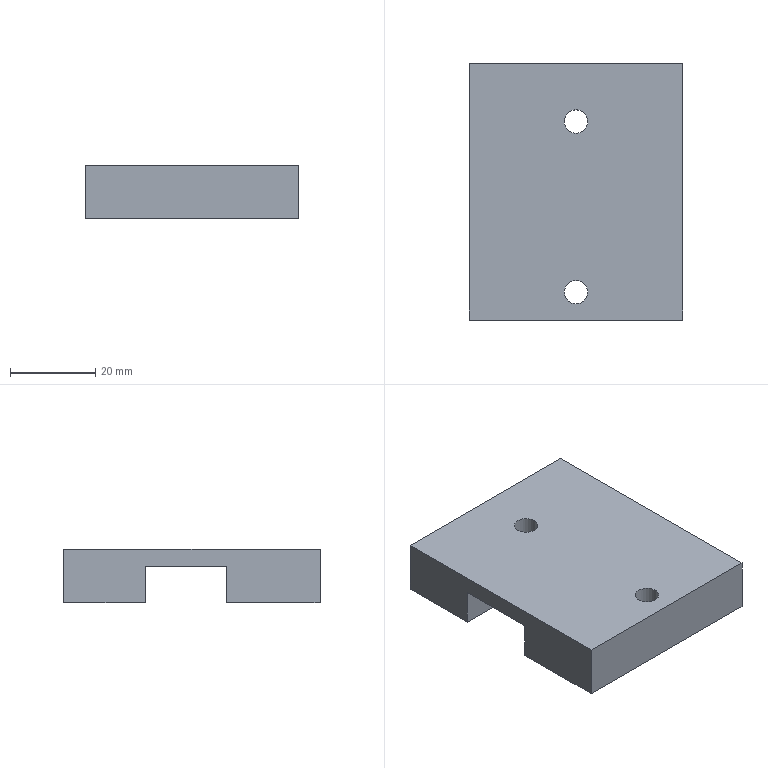Part | STEP file | 1 solid | 16 faces | box 50 x 60 x 12.5 mm | volume 28207 mm3 | plane 12 | cylinder 4 | commonest cylinder face diameters 5.5 x2 10 x2
STEP:
#1=CARTESIAN_POINT('',(0.,0.,0.));
#2=DIRECTION('',(0.,0.,1.));
#3=DIRECTION('',(1.,0.,0.));
#4=AXIS2_PLACEMENT_3D('',#1,#2,#3);
#5=CARTESIAN_POINT('',(-25.,0.,12.5));
#6=VERTEX_POINT('',#5);
#7=CARTESIAN_POINT('',(25.,0.,12.5));
#8=VERTEX_POINT('',#7);
#9=CARTESIAN_POINT('',(-25.,0.,12.5));
#10=DIRECTION('',(1.,0.,0.));
#11=VECTOR('',#10,1.);
#12=LINE('',#9,#11);
#13=CARTESIAN_POINT('',(0.,0.,12.5));
#14=DIRECTION('',(0.,0.,1.));
#15=DIRECTION('',(1.,0.,0.));
#16=AXIS2_PLACEMENT_3D('',#13,#14,#15);
#17=PLANE('',#16);
#18=CARTESIAN_POINT('',(-25.,0.));
#19=DIRECTION('',(1.,0.));
#20=VECTOR('',#19,1.);
#21=LINE('',#18,#20);
#22=(GEOMETRIC_REPRESENTATION_CONTEXT(2)PARAMETRIC_REPRESENTATION_CONTEXT()REPRESENTATION_CONTEXT('',''));
#23=DEFINITIONAL_REPRESENTATION('',(#21),#22);
#24=PCURVE('',#17,#23);
#25=CARTESIAN_POINT('',(0.,0.,0.));
#26=DIRECTION('',(0.,-1.,0.));
#27=DIRECTION('',(0.,0.,-1.));
#28=AXIS2_PLACEMENT_3D('',#25,#26,#27);
#29=PLANE('',#28);
#30=CARTESIAN_POINT('',(-12.5,-25.));
#31=DIRECTION('',(0.,1.));
#32=VECTOR('',#31,1.);
#33=LINE('',#30,#32);
#34=(GEOMETRIC_REPRESENTATION_CONTEXT(2)PARAMETRIC_REPRESENTATION_CONTEXT()REPRESENTATION_CONTEXT('',''));
#35=DEFINITIONAL_REPRESENTATION('',(#33),#34);
#36=PCURVE('',#29,#35);
#37=SURFACE_CURVE('',#12,(#24,#36),.PCURVE_S1.);
#38=EDGE_CURVE('',#6,#8,#37,.T.);
#39=ORIENTED_EDGE('',*,*,#38,.T.);
#40=CARTESIAN_POINT('',(25.,60.,12.5));
#41=VERTEX_POINT('',#40);
#42=CARTESIAN_POINT('',(25.,60.,12.5));
#43=DIRECTION('',(0.,-1.,0.));
#44=VECTOR('',#43,1.);
#45=LINE('',#42,#44);
#46=CARTESIAN_POINT('',(25.,60.));
#47=DIRECTION('',(0.,-1.));
#48=VECTOR('',#47,1.);
#49=LINE('',#46,#48);
#50=(GEOMETRIC_REPRESENTATION_CONTEXT(2)PARAMETRIC_REPRESENTATION_CONTEXT()REPRESENTATION_CONTEXT('',''));
#51=DEFINITIONAL_REPRESENTATION('',(#49),#50);
#52=PCURVE('',#17,#51);
#53=CARTESIAN_POINT('',(25.,0.,0.));
#54=DIRECTION('',(1.,0.,0.));
#55=DIRECTION('',(0.,0.,-1.));
#56=AXIS2_PLACEMENT_3D('',#53,#54,#55);
#57=PLANE('',#56);
#58=CARTESIAN_POINT('',(-12.5,60.));
#59=DIRECTION('',(0.,-1.));
#60=VECTOR('',#59,1.);
#61=LINE('',#58,#60);
#62=(GEOMETRIC_REPRESENTATION_CONTEXT(2)PARAMETRIC_REPRESENTATION_CONTEXT()REPRESENTATION_CONTEXT('',''));
#63=DEFINITIONAL_REPRESENTATION('',(#61),#62);
#64=PCURVE('',#57,#63);
#65=SURFACE_CURVE('',#45,(#52,#64),.PCURVE_S1.);
#66=EDGE_CURVE('',#41,#8,#65,.T.);
#67=ORIENTED_EDGE('',*,*,#66,.F.);
#68=CARTESIAN_POINT('',(-25.,60.,12.5));
#69=VERTEX_POINT('',#68);
#70=CARTESIAN_POINT('',(-25.,60.,12.5));
#71=DIRECTION('',(1.,0.,0.));
#72=VECTOR('',#71,1.);
#73=LINE('',#70,#72);
#74=CARTESIAN_POINT('',(-25.,60.));
#75=DIRECTION('',(1.,0.));
#76=VECTOR('',#75,1.);
#77=LINE('',#74,#76);
#78=(GEOMETRIC_REPRESENTATION_CONTEXT(2)PARAMETRIC_REPRESENTATION_CONTEXT()REPRESENTATION_CONTEXT('',''));
#79=DEFINITIONAL_REPRESENTATION('',(#77),#78);
#80=PCURVE('',#17,#79);
#81=CARTESIAN_POINT('',(0.,60.,0.));
#82=DIRECTION('',(0.,1.,0.));
#83=DIRECTION('',(0.,0.,1.));
#84=AXIS2_PLACEMENT_3D('',#81,#82,#83);
#85=PLANE('',#84);
#86=CARTESIAN_POINT('',(12.5,-25.));
#87=DIRECTION('',(0.,1.));
#88=VECTOR('',#87,1.);
#89=LINE('',#86,#88);
#90=(GEOMETRIC_REPRESENTATION_CONTEXT(2)PARAMETRIC_REPRESENTATION_CONTEXT()REPRESENTATION_CONTEXT('',''));
#91=DEFINITIONAL_REPRESENTATION('',(#89),#90);
#92=PCURVE('',#85,#91);
#93=SURFACE_CURVE('',#73,(#80,#92),.PCURVE_S1.);
#94=EDGE_CURVE('',#69,#41,#93,.T.);
#95=ORIENTED_EDGE('',*,*,#94,.F.);
#96=CARTESIAN_POINT('',(-25.,60.,12.5));
#97=DIRECTION('',(0.,-1.,0.));
#98=VECTOR('',#97,1.);
#99=LINE('',#96,#98);
#100=CARTESIAN_POINT('',(-25.,60.));
#101=DIRECTION('',(0.,-1.));
#102=VECTOR('',#101,1.);
#103=LINE('',#100,#102);
#104=(GEOMETRIC_REPRESENTATION_CONTEXT(2)PARAMETRIC_REPRESENTATION_CONTEXT()REPRESENTATION_CONTEXT('',''));
#105=DEFINITIONAL_REPRESENTATION('',(#103),#104);
#106=PCURVE('',#17,#105);
#107=CARTESIAN_POINT('',(-25.,0.,0.));
#108=DIRECTION('',(1.,0.,0.));
#109=DIRECTION('',(0.,0.,-1.));
#110=AXIS2_PLACEMENT_3D('',#107,#108,#109);
#111=PLANE('',#110);
#112=CARTESIAN_POINT('',(-12.5,60.));
#113=DIRECTION('',(0.,-1.));
#114=VECTOR('',#113,1.);
#115=LINE('',#112,#114);
#116=(GEOMETRIC_REPRESENTATION_CONTEXT(2)PARAMETRIC_REPRESENTATION_CONTEXT()REPRESENTATION_CONTEXT('',''));
#117=DEFINITIONAL_REPRESENTATION('',(#115),#116);
#118=PCURVE('',#111,#117);
#119=SURFACE_CURVE('',#99,(#106,#118),.PCURVE_S1.);
#120=EDGE_CURVE('',#69,#6,#119,.T.);
#121=ORIENTED_EDGE('',*,*,#120,.T.);
#122=EDGE_LOOP('',(#39,#67,#95,#121));
#123=FACE_BOUND('',#122,.T.);
#124=CARTESIAN_POINT('',(0.,43.75,12.5));
#125=VERTEX_POINT('',#124);
#126=CARTESIAN_POINT('',(0.,46.5,12.5));
#127=DIRECTION('',(0.,0.,1.));
#128=DIRECTION('',(1.,0.,0.));
#129=AXIS2_PLACEMENT_3D('',#126,#127,#128);
#130=CIRCLE('',#129,2.75);
#131=CARTESIAN_POINT('',(0.,46.5));
#132=DIRECTION('',(1.,0.));
#133=AXIS2_PLACEMENT_2D('',#131,#132);
#134=CIRCLE('',#133,2.75);
#135=(GEOMETRIC_REPRESENTATION_CONTEXT(2)PARAMETRIC_REPRESENTATION_CONTEXT()REPRESENTATION_CONTEXT('',''));
#136=DEFINITIONAL_REPRESENTATION('',(#134),#135);
#137=PCURVE('',#17,#136);
#138=CARTESIAN_POINT('',(0.,46.5,9.1));
#139=DIRECTION('',(0.,0.,1.));
#140=DIRECTION('',(0.,-1.,0.));
#141=AXIS2_PLACEMENT_3D('',#138,#139,#140);
#142=CYLINDRICAL_SURFACE('',#141,2.75);
#143=CARTESIAN_POINT('',(-4.712,3.4));
#144=DIRECTION('',(1.,0.));
#145=VECTOR('',#144,1.);
#146=LINE('',#143,#145);
#147=(GEOMETRIC_REPRESENTATION_CONTEXT(2)PARAMETRIC_REPRESENTATION_CONTEXT()REPRESENTATION_CONTEXT('',''));
#148=DEFINITIONAL_REPRESENTATION('',(#146),#147);
#149=PCURVE('',#142,#148);
#150=SURFACE_CURVE('',#130,(#137,#149),.PCURVE_S1.);
#151=EDGE_CURVE('',#125,#125,#150,.T.);
#152=ORIENTED_EDGE('',*,*,#151,.F.);
#153=EDGE_LOOP('',(#152));
#154=FACE_BOUND('',#153,.T.);
#155=CARTESIAN_POINT('',(0.,3.75,12.5));
#156=VERTEX_POINT('',#155);
#157=CARTESIAN_POINT('',(0.,6.5,12.5));
#158=DIRECTION('',(0.,0.,1.));
#159=DIRECTION('',(1.,0.,0.));
#160=AXIS2_PLACEMENT_3D('',#157,#158,#159);
#161=CIRCLE('',#160,2.75);
#162=CARTESIAN_POINT('',(0.,6.5));
#163=DIRECTION('',(1.,0.));
#164=AXIS2_PLACEMENT_2D('',#162,#163);
#165=CIRCLE('',#164,2.75);
#166=(GEOMETRIC_REPRESENTATION_CONTEXT(2)PARAMETRIC_REPRESENTATION_CONTEXT()REPRESENTATION_CONTEXT('',''));
#167=DEFINITIONAL_REPRESENTATION('',(#165),#166);
#168=PCURVE('',#17,#167);
#169=CARTESIAN_POINT('',(0.,6.5,9.1));
#170=DIRECTION('',(0.,0.,1.));
#171=DIRECTION('',(0.,-1.,0.));
#172=AXIS2_PLACEMENT_3D('',#169,#170,#171);
#173=CYLINDRICAL_SURFACE('',#172,2.75);
#174=CARTESIAN_POINT('',(-4.712,3.4));
#175=DIRECTION('',(1.,0.));
#176=VECTOR('',#175,1.);
#177=LINE('',#174,#176);
#178=(GEOMETRIC_REPRESENTATION_CONTEXT(2)PARAMETRIC_REPRESENTATION_CONTEXT()REPRESENTATION_CONTEXT('',''));
#179=DEFINITIONAL_REPRESENTATION('',(#177),#178);
#180=PCURVE('',#173,#179);
#181=SURFACE_CURVE('',#161,(#168,#180),.PCURVE_S1.);
#182=EDGE_CURVE('',#156,#156,#181,.T.);
#183=ORIENTED_EDGE('',*,*,#182,.F.);
#184=EDGE_LOOP('',(#183));
#185=FACE_BOUND('',#184,.T.);
#186=ADVANCED_FACE('',(#123,#154,#185),#17,.T.);
#187=CARTESIAN_POINT('',(25.,0.,0.));
#188=VERTEX_POINT('',#187);
#189=CARTESIAN_POINT('',(-25.,0.,0.));
#190=VERTEX_POINT('',#189);
#191=CARTESIAN_POINT('',(25.,0.,0.));
#192=DIRECTION('',(-1.,0.,0.));
#193=VECTOR('',#192,1.);
#194=LINE('',#191,#193);
#195=CARTESIAN_POINT('',(0.,25.));
#196=DIRECTION('',(0.,-1.));
#197=VECTOR('',#196,1.);
#198=LINE('',#195,#197);
#199=(GEOMETRIC_REPRESENTATION_CONTEXT(2)PARAMETRIC_REPRESENTATION_CONTEXT()REPRESENTATION_CONTEXT('',''));
#200=DEFINITIONAL_REPRESENTATION('',(#198),#199);
#201=PCURVE('',#29,#200);
#202=CARTESIAN_POINT('',(0.,22.,0.));
#203=DIRECTION('',(0.,0.,-1.));
#204=DIRECTION('',(-1.,0.,0.));
#205=AXIS2_PLACEMENT_3D('',#202,#203,#204);
#206=PLANE('',#205);
#207=CARTESIAN_POINT('',(-25.,-22.));
#208=DIRECTION('',(1.,0.));
#209=VECTOR('',#208,1.);
#210=LINE('',#207,#209);
#211=(GEOMETRIC_REPRESENTATION_CONTEXT(2)PARAMETRIC_REPRESENTATION_CONTEXT()REPRESENTATION_CONTEXT('',''));
#212=DEFINITIONAL_REPRESENTATION('',(#210),#211);
#213=PCURVE('',#206,#212);
#214=SURFACE_CURVE('',#194,(#201,#213),.PCURVE_S1.);
#215=EDGE_CURVE('',#188,#190,#214,.T.);
#216=ORIENTED_EDGE('',*,*,#215,.F.);
#217=CARTESIAN_POINT('',(25.,0.,12.5));
#218=DIRECTION('',(0.,0.,-1.));
#219=VECTOR('',#218,1.);
#220=LINE('',#217,#219);
#221=CARTESIAN_POINT('',(-12.5,25.));
#222=DIRECTION('',(1.,0.));
#223=VECTOR('',#222,1.);
#224=LINE('',#221,#223);
#225=(GEOMETRIC_REPRESENTATION_CONTEXT(2)PARAMETRIC_REPRESENTATION_CONTEXT()REPRESENTATION_CONTEXT('',''));
#226=DEFINITIONAL_REPRESENTATION('',(#224),#225);
#227=PCURVE('',#29,#226);
#228=CARTESIAN_POINT('',(-12.5,0.));
#229=DIRECTION('',(1.,0.));
#230=VECTOR('',#229,1.);
#231=LINE('',#228,#230);
#232=(GEOMETRIC_REPRESENTATION_CONTEXT(2)PARAMETRIC_REPRESENTATION_CONTEXT()REPRESENTATION_CONTEXT('',''));
#233=DEFINITIONAL_REPRESENTATION('',(#231),#232);
#234=PCURVE('',#57,#233);
#235=SURFACE_CURVE('',#220,(#227,#234),.PCURVE_S1.);
#236=EDGE_CURVE('',#8,#188,#235,.T.);
#237=ORIENTED_EDGE('',*,*,#236,.F.);
#238=ORIENTED_EDGE('',*,*,#38,.F.);
#239=CARTESIAN_POINT('',(-25.,0.,12.5));
#240=DIRECTION('',(0.,0.,-1.));
#241=VECTOR('',#240,1.);
#242=LINE('',#239,#241);
#243=CARTESIAN_POINT('',(-12.5,-25.));
#244=DIRECTION('',(1.,0.));
#245=VECTOR('',#244,1.);
#246=LINE('',#243,#245);
#247=(GEOMETRIC_REPRESENTATION_CONTEXT(2)PARAMETRIC_REPRESENTATION_CONTEXT()REPRESENTATION_CONTEXT('',''));
#248=DEFINITIONAL_REPRESENTATION('',(#246),#247);
#249=PCURVE('',#29,#248);
#250=CARTESIAN_POINT('',(-12.5,0.));
#251=DIRECTION('',(1.,0.));
#252=VECTOR('',#251,1.);
#253=LINE('',#250,#252);
#254=(GEOMETRIC_REPRESENTATION_CONTEXT(2)PARAMETRIC_REPRESENTATION_CONTEXT()REPRESENTATION_CONTEXT('',''));
#255=DEFINITIONAL_REPRESENTATION('',(#253),#254);
#256=PCURVE('',#111,#255);
#257=SURFACE_CURVE('',#242,(#249,#256),.PCURVE_S1.);
#258=EDGE_CURVE('',#6,#190,#257,.T.);
#259=ORIENTED_EDGE('',*,*,#258,.T.);
#260=EDGE_LOOP('',(#216,#237,#238,#259));
#261=FACE_BOUND('',#260,.T.);
#262=ADVANCED_FACE('',(#261),#29,.T.);
#263=ORIENTED_EDGE('',*,*,#236,.T.);
#264=CARTESIAN_POINT('',(25.,22.,0.));
#265=VERTEX_POINT('',#264);
#266=CARTESIAN_POINT('',(25.,0.,0.));
#267=DIRECTION('',(0.,1.,0.));
#268=VECTOR('',#267,1.);
#269=LINE('',#266,#268);
#270=CARTESIAN_POINT('',(0.,0.));
#271=DIRECTION('',(0.,1.));
#272=VECTOR('',#271,1.);
#273=LINE('',#270,#272);
#274=(GEOMETRIC_REPRESENTATION_CONTEXT(2)PARAMETRIC_REPRESENTATION_CONTEXT()REPRESENTATION_CONTEXT('',''));
#275=DEFINITIONAL_REPRESENTATION('',(#273),#274);
#276=PCURVE('',#57,#275);
#277=CARTESIAN_POINT('',(-25.,-22.));
#278=DIRECTION('',(0.,1.));
#279=VECTOR('',#278,1.);
#280=LINE('',#277,#279);
#281=(GEOMETRIC_REPRESENTATION_CONTEXT(2)PARAMETRIC_REPRESENTATION_CONTEXT()REPRESENTATION_CONTEXT('',''));
#282=DEFINITIONAL_REPRESENTATION('',(#280),#281);
#283=PCURVE('',#206,#282);
#284=SURFACE_CURVE('',#269,(#276,#283),.PCURVE_S1.);
#285=EDGE_CURVE('',#188,#265,#284,.T.);
#286=ORIENTED_EDGE('',*,*,#285,.T.);
#287=CARTESIAN_POINT('',(25.,22.,8.5));
#288=VERTEX_POINT('',#287);
#289=CARTESIAN_POINT('',(25.,22.,0.));
#290=DIRECTION('',(0.,0.,1.));
#291=VECTOR('',#290,1.);
#292=LINE('',#289,#291);
#293=CARTESIAN_POINT('',(0.,22.));
#294=DIRECTION('',(-1.,0.));
#295=VECTOR('',#294,1.);
#296=LINE('',#293,#295);
#297=(GEOMETRIC_REPRESENTATION_CONTEXT(2)PARAMETRIC_REPRESENTATION_CONTEXT()REPRESENTATION_CONTEXT('',''));
#298=DEFINITIONAL_REPRESENTATION('',(#296),#297);
#299=PCURVE('',#57,#298);
#300=CARTESIAN_POINT('',(0.,22.,0.));
#301=DIRECTION('',(0.,1.,0.));
#302=DIRECTION('',(0.,0.,1.));
#303=AXIS2_PLACEMENT_3D('',#300,#301,#302);
#304=PLANE('',#303);
#305=CARTESIAN_POINT('',(0.,25.));
#306=DIRECTION('',(1.,0.));
#307=VECTOR('',#306,1.);
#308=LINE('',#305,#307);
#309=(GEOMETRIC_REPRESENTATION_CONTEXT(2)PARAMETRIC_REPRESENTATION_CONTEXT()REPRESENTATION_CONTEXT('',''));
#310=DEFINITIONAL_REPRESENTATION('',(#308),#309);
#311=PCURVE('',#304,#310);
#312=SURFACE_CURVE('',#292,(#299,#311),.PCURVE_S1.);
#313=EDGE_CURVE('',#265,#288,#312,.T.);
#314=ORIENTED_EDGE('',*,*,#313,.T.);
#315=CARTESIAN_POINT('',(25.,41.,8.5));
#316=VERTEX_POINT('',#315);
#317=CARTESIAN_POINT('',(25.,22.,8.5));
#318=DIRECTION('',(0.,1.,0.));
#319=VECTOR('',#318,1.);
#320=LINE('',#317,#319);
#321=CARTESIAN_POINT('',(-8.5,22.));
#322=DIRECTION('',(0.,1.));
#323=VECTOR('',#322,1.);
#324=LINE('',#321,#323);
#325=(GEOMETRIC_REPRESENTATION_CONTEXT(2)PARAMETRIC_REPRESENTATION_CONTEXT()REPRESENTATION_CONTEXT('',''));
#326=DEFINITIONAL_REPRESENTATION('',(#324),#325);
#327=PCURVE('',#57,#326);
#328=CARTESIAN_POINT('',(0.,22.,8.5));
#329=DIRECTION('',(0.,0.,-1.));
#330=DIRECTION('',(-1.,0.,0.));
#331=AXIS2_PLACEMENT_3D('',#328,#329,#330);
#332=PLANE('',#331);
#333=CARTESIAN_POINT('',(-25.,0.));
#334=DIRECTION('',(0.,1.));
#335=VECTOR('',#334,1.);
#336=LINE('',#333,#335);
#337=(GEOMETRIC_REPRESENTATION_CONTEXT(2)PARAMETRIC_REPRESENTATION_CONTEXT()REPRESENTATION_CONTEXT('',''));
#338=DEFINITIONAL_REPRESENTATION('',(#336),#337);
#339=PCURVE('',#332,#338);
#340=SURFACE_CURVE('',#320,(#327,#339),.PCURVE_S1.);
#341=EDGE_CURVE('',#288,#316,#340,.T.);
#342=ORIENTED_EDGE('',*,*,#341,.T.);
#343=CARTESIAN_POINT('',(25.,41.,0.));
#344=VERTEX_POINT('',#343);
#345=CARTESIAN_POINT('',(25.,41.,8.5));
#346=DIRECTION('',(0.,0.,-1.));
#347=VECTOR('',#346,1.);
#348=LINE('',#345,#347);
#349=CARTESIAN_POINT('',(-8.5,41.));
#350=DIRECTION('',(1.,0.));
#351=VECTOR('',#350,1.);
#352=LINE('',#349,#351);
#353=(GEOMETRIC_REPRESENTATION_CONTEXT(2)PARAMETRIC_REPRESENTATION_CONTEXT()REPRESENTATION_CONTEXT('',''));
#354=DEFINITIONAL_REPRESENTATION('',(#352),#353);
#355=PCURVE('',#57,#354);
#356=CARTESIAN_POINT('',(0.,41.,8.5));
#357=DIRECTION('',(0.,-1.,0.));
#358=DIRECTION('',(0.,0.,-1.));
#359=AXIS2_PLACEMENT_3D('',#356,#357,#358);
#360=PLANE('',#359);
#361=CARTESIAN_POINT('',(0.,25.));
#362=DIRECTION('',(1.,0.));
#363=VECTOR('',#362,1.);
#364=LINE('',#361,#363);
#365=(GEOMETRIC_REPRESENTATION_CONTEXT(2)PARAMETRIC_REPRESENTATION_CONTEXT()REPRESENTATION_CONTEXT('',''));
#366=DEFINITIONAL_REPRESENTATION('',(#364),#365);
#367=PCURVE('',#360,#366);
#368=SURFACE_CURVE('',#348,(#355,#367),.PCURVE_S1.);
#369=EDGE_CURVE('',#316,#344,#368,.T.);
#370=ORIENTED_EDGE('',*,*,#369,.T.);
#371=CARTESIAN_POINT('',(25.,60.,0.));
#372=VERTEX_POINT('',#371);
#373=CARTESIAN_POINT('',(25.,41.,0.));
#374=DIRECTION('',(0.,1.,0.));
#375=VECTOR('',#374,1.);
#376=LINE('',#373,#375);
#377=CARTESIAN_POINT('',(0.,41.));
#378=DIRECTION('',(0.,1.));
#379=VECTOR('',#378,1.);
#380=LINE('',#377,#379);
#381=(GEOMETRIC_REPRESENTATION_CONTEXT(2)PARAMETRIC_REPRESENTATION_CONTEXT()REPRESENTATION_CONTEXT('',''));
#382=DEFINITIONAL_REPRESENTATION('',(#380),#381);
#383=PCURVE('',#57,#382);
#384=CARTESIAN_POINT('',(0.,41.,0.));
#385=DIRECTION('',(0.,0.,-1.));
#386=DIRECTION('',(-1.,0.,0.));
#387=AXIS2_PLACEMENT_3D('',#384,#385,#386);
#388=PLANE('',#387);
#389=CARTESIAN_POINT('',(-25.,0.));
#390=DIRECTION('',(0.,1.));
#391=VECTOR('',#390,1.);
#392=LINE('',#389,#391);
#393=(GEOMETRIC_REPRESENTATION_CONTEXT(2)PARAMETRIC_REPRESENTATION_CONTEXT()REPRESENTATION_CONTEXT('',''));
#394=DEFINITIONAL_REPRESENTATION('',(#392),#393);
#395=PCURVE('',#388,#394);
#396=SURFACE_CURVE('',#376,(#383,#395),.PCURVE_S1.);
#397=EDGE_CURVE('',#344,#372,#396,.T.);
#398=ORIENTED_EDGE('',*,*,#397,.T.);
#399=CARTESIAN_POINT('',(25.,60.,0.));
#400=DIRECTION('',(0.,0.,1.));
#401=VECTOR('',#400,1.);
#402=LINE('',#399,#401);
#403=CARTESIAN_POINT('',(0.,60.));
#404=DIRECTION('',(-1.,0.));
#405=VECTOR('',#404,1.);
#406=LINE('',#403,#405);
#407=(GEOMETRIC_REPRESENTATION_CONTEXT(2)PARAMETRIC_REPRESENTATION_CONTEXT()REPRESENTATION_CONTEXT('',''));
#408=DEFINITIONAL_REPRESENTATION('',(#406),#407);
#409=PCURVE('',#57,#408);
#410=CARTESIAN_POINT('',(0.,25.));
#411=DIRECTION('',(1.,0.));
#412=VECTOR('',#411,1.);
#413=LINE('',#410,#412);
#414=(GEOMETRIC_REPRESENTATION_CONTEXT(2)PARAMETRIC_REPRESENTATION_CONTEXT()REPRESENTATION_CONTEXT('',''));
#415=DEFINITIONAL_REPRESENTATION('',(#413),#414);
#416=PCURVE('',#85,#415);
#417=SURFACE_CURVE('',#402,(#409,#416),.PCURVE_S1.);
#418=EDGE_CURVE('',#372,#41,#417,.T.);
#419=ORIENTED_EDGE('',*,*,#418,.T.);
#420=ORIENTED_EDGE('',*,*,#66,.T.);
#421=EDGE_LOOP('',(#263,#286,#314,#342,#370,#398,#419,#420));
#422=FACE_BOUND('',#421,.T.);
#423=ADVANCED_FACE('',(#422),#57,.T.);
#424=CARTESIAN_POINT('',(-25.,60.,0.));
#425=VERTEX_POINT('',#424);
#426=CARTESIAN_POINT('',(25.,60.,0.));
#427=DIRECTION('',(-1.,0.,0.));
#428=VECTOR('',#427,1.);
#429=LINE('',#426,#428);
#430=CARTESIAN_POINT('',(0.,25.));
#431=DIRECTION('',(0.,-1.));
#432=VECTOR('',#431,1.);
#433=LINE('',#430,#432);
#434=(GEOMETRIC_REPRESENTATION_CONTEXT(2)PARAMETRIC_REPRESENTATION_CONTEXT()REPRESENTATION_CONTEXT('',''));
#435=DEFINITIONAL_REPRESENTATION('',(#433),#434);
#436=PCURVE('',#85,#435);
#437=CARTESIAN_POINT('',(-25.,19.));
#438=DIRECTION('',(1.,0.));
#439=VECTOR('',#438,1.);
#440=LINE('',#437,#439);
#441=(GEOMETRIC_REPRESENTATION_CONTEXT(2)PARAMETRIC_REPRESENTATION_CONTEXT()REPRESENTATION_CONTEXT('',''));
#442=DEFINITIONAL_REPRESENTATION('',(#440),#441);
#443=PCURVE('',#388,#442);
#444=SURFACE_CURVE('',#429,(#436,#443),.PCURVE_S1.);
#445=EDGE_CURVE('',#372,#425,#444,.T.);
#446=ORIENTED_EDGE('',*,*,#445,.T.);
#447=CARTESIAN_POINT('',(-25.,60.,0.));
#448=DIRECTION('',(0.,0.,1.));
#449=VECTOR('',#448,1.);
#450=LINE('',#447,#449);
#451=CARTESIAN_POINT('',(0.,-25.));
#452=DIRECTION('',(1.,0.));
#453=VECTOR('',#452,1.);
#454=LINE('',#451,#453);
#455=(GEOMETRIC_REPRESENTATION_CONTEXT(2)PARAMETRIC_REPRESENTATION_CONTEXT()REPRESENTATION_CONTEXT('',''));
#456=DEFINITIONAL_REPRESENTATION('',(#454),#455);
#457=PCURVE('',#85,#456);
#458=CARTESIAN_POINT('',(0.,60.));
#459=DIRECTION('',(-1.,0.));
#460=VECTOR('',#459,1.);
#461=LINE('',#458,#460);
#462=(GEOMETRIC_REPRESENTATION_CONTEXT(2)PARAMETRIC_REPRESENTATION_CONTEXT()REPRESENTATION_CONTEXT('',''));
#463=DEFINITIONAL_REPRESENTATION('',(#461),#462);
#464=PCURVE('',#111,#463);
#465=SURFACE_CURVE('',#450,(#457,#464),.PCURVE_S1.);
#466=EDGE_CURVE('',#425,#69,#465,.T.);
#467=ORIENTED_EDGE('',*,*,#466,.T.);
#468=ORIENTED_EDGE('',*,*,#94,.T.);
#469=ORIENTED_EDGE('',*,*,#418,.F.);
#470=EDGE_LOOP('',(#446,#467,#468,#469));
#471=FACE_BOUND('',#470,.T.);
#472=ADVANCED_FACE('',(#471),#85,.T.);
#473=ORIENTED_EDGE('',*,*,#120,.F.);
#474=ORIENTED_EDGE('',*,*,#466,.F.);
#475=CARTESIAN_POINT('',(-25.,41.,0.));
#476=VERTEX_POINT('',#475);
#477=CARTESIAN_POINT('',(-25.,41.,0.));
#478=DIRECTION('',(0.,1.,0.));
#479=VECTOR('',#478,1.);
#480=LINE('',#477,#479);
#481=CARTESIAN_POINT('',(0.,41.));
#482=DIRECTION('',(0.,1.));
#483=VECTOR('',#482,1.);
#484=LINE('',#481,#483);
#485=(GEOMETRIC_REPRESENTATION_CONTEXT(2)PARAMETRIC_REPRESENTATION_CONTEXT()REPRESENTATION_CONTEXT('',''));
#486=DEFINITIONAL_REPRESENTATION('',(#484),#485);
#487=PCURVE('',#111,#486);
#488=CARTESIAN_POINT('',(25.,0.));
#489=DIRECTION('',(0.,1.));
#490=VECTOR('',#489,1.);
#491=LINE('',#488,#490);
#492=(GEOMETRIC_REPRESENTATION_CONTEXT(2)PARAMETRIC_REPRESENTATION_CONTEXT()REPRESENTATION_CONTEXT('',''));
#493=DEFINITIONAL_REPRESENTATION('',(#491),#492);
#494=PCURVE('',#388,#493);
#495=SURFACE_CURVE('',#480,(#487,#494),.PCURVE_S1.);
#496=EDGE_CURVE('',#476,#425,#495,.T.);
#497=ORIENTED_EDGE('',*,*,#496,.F.);
#498=CARTESIAN_POINT('',(-25.,41.,8.5));
#499=VERTEX_POINT('',#498);
#500=CARTESIAN_POINT('',(-25.,41.,8.5));
#501=DIRECTION('',(0.,0.,-1.));
#502=VECTOR('',#501,1.);
#503=LINE('',#500,#502);
#504=CARTESIAN_POINT('',(-8.5,41.));
#505=DIRECTION('',(1.,0.));
#506=VECTOR('',#505,1.);
#507=LINE('',#504,#506);
#508=(GEOMETRIC_REPRESENTATION_CONTEXT(2)PARAMETRIC_REPRESENTATION_CONTEXT()REPRESENTATION_CONTEXT('',''));
#509=DEFINITIONAL_REPRESENTATION('',(#507),#508);
#510=PCURVE('',#111,#509);
#511=CARTESIAN_POINT('',(0.,-25.));
#512=DIRECTION('',(1.,0.));
#513=VECTOR('',#512,1.);
#514=LINE('',#511,#513);
#515=(GEOMETRIC_REPRESENTATION_CONTEXT(2)PARAMETRIC_REPRESENTATION_CONTEXT()REPRESENTATION_CONTEXT('',''));
#516=DEFINITIONAL_REPRESENTATION('',(#514),#515);
#517=PCURVE('',#360,#516);
#518=SURFACE_CURVE('',#503,(#510,#517),.PCURVE_S1.);
#519=EDGE_CURVE('',#499,#476,#518,.T.);
#520=ORIENTED_EDGE('',*,*,#519,.F.);
#521=CARTESIAN_POINT('',(-25.,22.,8.5));
#522=VERTEX_POINT('',#521);
#523=CARTESIAN_POINT('',(-25.,22.,8.5));
#524=DIRECTION('',(0.,1.,0.));
#525=VECTOR('',#524,1.);
#526=LINE('',#523,#525);
#527=CARTESIAN_POINT('',(-8.5,22.));
#528=DIRECTION('',(0.,1.));
#529=VECTOR('',#528,1.);
#530=LINE('',#527,#529);
#531=(GEOMETRIC_REPRESENTATION_CONTEXT(2)PARAMETRIC_REPRESENTATION_CONTEXT()REPRESENTATION_CONTEXT('',''));
#532=DEFINITIONAL_REPRESENTATION('',(#530),#531);
#533=PCURVE('',#111,#532);
#534=CARTESIAN_POINT('',(25.,0.));
#535=DIRECTION('',(0.,1.));
#536=VECTOR('',#535,1.);
#537=LINE('',#534,#536);
#538=(GEOMETRIC_REPRESENTATION_CONTEXT(2)PARAMETRIC_REPRESENTATION_CONTEXT()REPRESENTATION_CONTEXT('',''));
#539=DEFINITIONAL_REPRESENTATION('',(#537),#538);
#540=PCURVE('',#332,#539);
#541=SURFACE_CURVE('',#526,(#533,#540),.PCURVE_S1.);
#542=EDGE_CURVE('',#522,#499,#541,.T.);
#543=ORIENTED_EDGE('',*,*,#542,.F.);
#544=CARTESIAN_POINT('',(-25.,22.,0.));
#545=VERTEX_POINT('',#544);
#546=CARTESIAN_POINT('',(-25.,22.,0.));
#547=DIRECTION('',(0.,0.,1.));
#548=VECTOR('',#547,1.);
#549=LINE('',#546,#548);
#550=CARTESIAN_POINT('',(0.,22.));
#551=DIRECTION('',(-1.,0.));
#552=VECTOR('',#551,1.);
#553=LINE('',#550,#552);
#554=(GEOMETRIC_REPRESENTATION_CONTEXT(2)PARAMETRIC_REPRESENTATION_CONTEXT()REPRESENTATION_CONTEXT('',''));
#555=DEFINITIONAL_REPRESENTATION('',(#553),#554);
#556=PCURVE('',#111,#555);
#557=CARTESIAN_POINT('',(0.,-25.));
#558=DIRECTION('',(1.,0.));
#559=VECTOR('',#558,1.);
#560=LINE('',#557,#559);
#561=(GEOMETRIC_REPRESENTATION_CONTEXT(2)PARAMETRIC_REPRESENTATION_CONTEXT()REPRESENTATION_CONTEXT('',''));
#562=DEFINITIONAL_REPRESENTATION('',(#560),#561);
#563=PCURVE('',#304,#562);
#564=SURFACE_CURVE('',#549,(#556,#563),.PCURVE_S1.);
#565=EDGE_CURVE('',#545,#522,#564,.T.);
#566=ORIENTED_EDGE('',*,*,#565,.F.);
#567=CARTESIAN_POINT('',(-25.,0.,0.));
#568=DIRECTION('',(0.,1.,0.));
#569=VECTOR('',#568,1.);
#570=LINE('',#567,#569);
#571=CARTESIAN_POINT('',(0.,0.));
#572=DIRECTION('',(0.,1.));
#573=VECTOR('',#572,1.);
#574=LINE('',#571,#573);
#575=(GEOMETRIC_REPRESENTATION_CONTEXT(2)PARAMETRIC_REPRESENTATION_CONTEXT()REPRESENTATION_CONTEXT('',''));
#576=DEFINITIONAL_REPRESENTATION('',(#574),#575);
#577=PCURVE('',#111,#576);
#578=CARTESIAN_POINT('',(25.,-22.));
#579=DIRECTION('',(0.,1.));
#580=VECTOR('',#579,1.);
#581=LINE('',#578,#580);
#582=(GEOMETRIC_REPRESENTATION_CONTEXT(2)PARAMETRIC_REPRESENTATION_CONTEXT()REPRESENTATION_CONTEXT('',''));
#583=DEFINITIONAL_REPRESENTATION('',(#581),#582);
#584=PCURVE('',#206,#583);
#585=SURFACE_CURVE('',#570,(#577,#584),.PCURVE_S1.);
#586=EDGE_CURVE('',#190,#545,#585,.T.);
#587=ORIENTED_EDGE('',*,*,#586,.F.);
#588=ORIENTED_EDGE('',*,*,#258,.F.);
#589=EDGE_LOOP('',(#473,#474,#497,#520,#543,#566,#587,#588));
#590=FACE_BOUND('',#589,.T.);
#591=ADVANCED_FACE('',(#590),#111,.F.);
#592=ORIENTED_EDGE('',*,*,#151,.F.);
#593=CARTESIAN_POINT('',(0.,43.75,5.7));
#594=VERTEX_POINT('',#593);
#595=CARTESIAN_POINT('',(0.,43.75,5.7));
#596=CARTESIAN_POINT('',(0.,43.75,12.5));
#597=B_SPLINE_CURVE_WITH_KNOTS('',1,(#595,#596),.UNSPECIFIED.,.F.,.F.,(2,2),(-3.4,3.4),.PIECEWISE_BEZIER_KNOTS.);
#598=CARTESIAN_POINT('',(0.,0.));
#599=DIRECTION('',(0.,1.));
#600=VECTOR('',#599,1.);
#601=LINE('',#598,#600);
#602=(GEOMETRIC_REPRESENTATION_CONTEXT(2)PARAMETRIC_REPRESENTATION_CONTEXT()REPRESENTATION_CONTEXT('',''));
#603=DEFINITIONAL_REPRESENTATION('',(#601),#602);
#604=PCURVE('',#142,#603);
#605=CARTESIAN_POINT('',(6.283,0.));
#606=DIRECTION('',(0.,1.));
#607=VECTOR('',#606,1.);
#608=LINE('',#605,#607);
#609=(GEOMETRIC_REPRESENTATION_CONTEXT(2)PARAMETRIC_REPRESENTATION_CONTEXT()REPRESENTATION_CONTEXT('',''));
#610=DEFINITIONAL_REPRESENTATION('',(#608),#609);
#611=PCURVE('',#142,#610);
#612=SEAM_CURVE('',#597,(#604,#611),.PCURVE_S1.);
#613=EDGE_CURVE('',#594,#125,#612,.T.);
#614=ORIENTED_EDGE('',*,*,#613,.F.);
#615=CARTESIAN_POINT('',(0.,46.5,5.7));
#616=DIRECTION('',(0.,0.,1.));
#617=DIRECTION('',(1.,0.,0.));
#618=AXIS2_PLACEMENT_3D('',#615,#616,#617);
#619=CIRCLE('',#618,2.75);
#620=CARTESIAN_POINT('',(-4.712,-3.4));
#621=DIRECTION('',(1.,0.));
#622=VECTOR('',#621,1.);
#623=LINE('',#620,#622);
#624=(GEOMETRIC_REPRESENTATION_CONTEXT(2)PARAMETRIC_REPRESENTATION_CONTEXT()REPRESENTATION_CONTEXT('',''));
#625=DEFINITIONAL_REPRESENTATION('',(#623),#624);
#626=PCURVE('',#142,#625);
#627=CARTESIAN_POINT('',(0.,50.375,5.7));
#628=DIRECTION('',(0.,0.,-1.));
#629=DIRECTION('',(-1.,0.,0.));
#630=AXIS2_PLACEMENT_3D('',#627,#628,#629);
#631=PLANE('',#630);
#632=CARTESIAN_POINT('',(-2.75,-3.875));
#633=CARTESIAN_POINT('',(-2.75,0.8881));
#634=CARTESIAN_POINT('',(1.375,-1.493));
#635=CARTESIAN_POINT('',(5.5,-3.875));
#636=CARTESIAN_POINT('',(1.375,-6.257));
#637=CARTESIAN_POINT('',(-2.75,-8.638));
#638=CARTESIAN_POINT('',(-2.75,-3.875));
#639=(BOUNDED_CURVE()B_SPLINE_CURVE(2,(#632,#633,#634,#635,#636,#637,#638),.UNSPECIFIED.,.T.,.F.)B_SPLINE_CURVE_WITH_KNOTS((1,2,2,2,2,1),(-2.094,0.,2.094,4.189,6.283,8.378),.UNSPECIFIED.)CURVE()GEOMETRIC_REPRESENTATION_ITEM()RATIONAL_B_SPLINE_CURVE((1.,0.5,1.,0.5,1.,0.5,1.))REPRESENTATION_ITEM(''));
#640=(GEOMETRIC_REPRESENTATION_CONTEXT(2)PARAMETRIC_REPRESENTATION_CONTEXT()REPRESENTATION_CONTEXT('',''));
#641=DEFINITIONAL_REPRESENTATION('',(#639),#640);
#642=PCURVE('',#631,#641);
#643=SURFACE_CURVE('',#619,(#626,#642),.PCURVE_S1.);
#644=EDGE_CURVE('',#594,#594,#643,.T.);
#645=ORIENTED_EDGE('',*,*,#644,.T.);
#646=ORIENTED_EDGE('',*,*,#613,.T.);
#647=EDGE_LOOP('',(#592,#614,#645,#646));
#648=FACE_BOUND('',#647,.F.);
#649=ADVANCED_FACE('',(#648),#142,.F.);
#650=ORIENTED_EDGE('',*,*,#182,.F.);
#651=CARTESIAN_POINT('',(0.,3.75,5.7));
#652=VERTEX_POINT('',#651);
#653=CARTESIAN_POINT('',(0.,3.75,5.7));
#654=CARTESIAN_POINT('',(0.,3.75,12.5));
#655=B_SPLINE_CURVE_WITH_KNOTS('',1,(#653,#654),.UNSPECIFIED.,.F.,.F.,(2,2),(-3.4,3.4),.PIECEWISE_BEZIER_KNOTS.);
#656=CARTESIAN_POINT('',(0.,0.));
#657=DIRECTION('',(0.,1.));
#658=VECTOR('',#657,1.);
#659=LINE('',#656,#658);
#660=(GEOMETRIC_REPRESENTATION_CONTEXT(2)PARAMETRIC_REPRESENTATION_CONTEXT()REPRESENTATION_CONTEXT('',''));
#661=DEFINITIONAL_REPRESENTATION('',(#659),#660);
#662=PCURVE('',#173,#661);
#663=CARTESIAN_POINT('',(6.283,0.));
#664=DIRECTION('',(0.,1.));
#665=VECTOR('',#664,1.);
#666=LINE('',#663,#665);
#667=(GEOMETRIC_REPRESENTATION_CONTEXT(2)PARAMETRIC_REPRESENTATION_CONTEXT()REPRESENTATION_CONTEXT('',''));
#668=DEFINITIONAL_REPRESENTATION('',(#666),#667);
#669=PCURVE('',#173,#668);
#670=SEAM_CURVE('',#655,(#662,#669),.PCURVE_S1.);
#671=EDGE_CURVE('',#652,#156,#670,.T.);
#672=ORIENTED_EDGE('',*,*,#671,.F.);
#673=CARTESIAN_POINT('',(0.,6.5,5.7));
#674=DIRECTION('',(0.,0.,1.));
#675=DIRECTION('',(1.,0.,0.));
#676=AXIS2_PLACEMENT_3D('',#673,#674,#675);
#677=CIRCLE('',#676,2.75);
#678=CARTESIAN_POINT('',(-4.712,-3.4));
#679=DIRECTION('',(1.,0.));
#680=VECTOR('',#679,1.);
#681=LINE('',#678,#680);
#682=(GEOMETRIC_REPRESENTATION_CONTEXT(2)PARAMETRIC_REPRESENTATION_CONTEXT()REPRESENTATION_CONTEXT('',''));
#683=DEFINITIONAL_REPRESENTATION('',(#681),#682);
#684=PCURVE('',#173,#683);
#685=CARTESIAN_POINT('',(0.,10.375,5.7));
#686=DIRECTION('',(0.,0.,-1.));
#687=DIRECTION('',(-1.,0.,0.));
#688=AXIS2_PLACEMENT_3D('',#685,#686,#687);
#689=PLANE('',#688);
#690=CARTESIAN_POINT('',(-2.75,-3.875));
#691=CARTESIAN_POINT('',(-2.75,0.8881));
#692=CARTESIAN_POINT('',(1.375,-1.493));
#693=CARTESIAN_POINT('',(5.5,-3.875));
#694=CARTESIAN_POINT('',(1.375,-6.257));
#695=CARTESIAN_POINT('',(-2.75,-8.638));
#696=CARTESIAN_POINT('',(-2.75,-3.875));
#697=(BOUNDED_CURVE()B_SPLINE_CURVE(2,(#690,#691,#692,#693,#694,#695,#696),.UNSPECIFIED.,.T.,.F.)B_SPLINE_CURVE_WITH_KNOTS((1,2,2,2,2,1),(-2.094,0.,2.094,4.189,6.283,8.378),.UNSPECIFIED.)CURVE()GEOMETRIC_REPRESENTATION_ITEM()RATIONAL_B_SPLINE_CURVE((1.,0.5,1.,0.5,1.,0.5,1.))REPRESENTATION_ITEM(''));
#698=(GEOMETRIC_REPRESENTATION_CONTEXT(2)PARAMETRIC_REPRESENTATION_CONTEXT()REPRESENTATION_CONTEXT('',''));
#699=DEFINITIONAL_REPRESENTATION('',(#697),#698);
#700=PCURVE('',#689,#699);
#701=SURFACE_CURVE('',#677,(#684,#700),.PCURVE_S1.);
#702=EDGE_CURVE('',#652,#652,#701,.T.);
#703=ORIENTED_EDGE('',*,*,#702,.T.);
#704=ORIENTED_EDGE('',*,*,#671,.T.);
#705=EDGE_LOOP('',(#650,#672,#703,#704));
#706=FACE_BOUND('',#705,.F.);
#707=ADVANCED_FACE('',(#706),#173,.F.);
#708=CARTESIAN_POINT('',(-25.,22.,0.));
#709=DIRECTION('',(1.,0.,0.));
#710=VECTOR('',#709,1.);
#711=LINE('',#708,#710);
#712=CARTESIAN_POINT('',(25.,0.));
#713=DIRECTION('',(-1.,0.));
#714=VECTOR('',#713,1.);
#715=LINE('',#712,#714);
#716=(GEOMETRIC_REPRESENTATION_CONTEXT(2)PARAMETRIC_REPRESENTATION_CONTEXT()REPRESENTATION_CONTEXT('',''));
#717=DEFINITIONAL_REPRESENTATION('',(#715),#716);
#718=PCURVE('',#206,#717);
#719=CARTESIAN_POINT('',(0.,-25.));
#720=DIRECTION('',(0.,1.));
#721=VECTOR('',#720,1.);
#722=LINE('',#719,#721);
#723=(GEOMETRIC_REPRESENTATION_CONTEXT(2)PARAMETRIC_REPRESENTATION_CONTEXT()REPRESENTATION_CONTEXT('',''));
#724=DEFINITIONAL_REPRESENTATION('',(#722),#723);
#725=PCURVE('',#304,#724);
#726=SURFACE_CURVE('',#711,(#718,#725),.PCURVE_S1.);
#727=EDGE_CURVE('',#545,#265,#726,.T.);
#728=ORIENTED_EDGE('',*,*,#727,.T.);
#729=ORIENTED_EDGE('',*,*,#285,.F.);
#730=ORIENTED_EDGE('',*,*,#215,.T.);
#731=ORIENTED_EDGE('',*,*,#586,.T.);
#732=EDGE_LOOP('',(#728,#729,#730,#731));
#733=FACE_BOUND('',#732,.T.);
#734=CARTESIAN_POINT('',(0.,11.5,0.));
#735=VERTEX_POINT('',#734);
#736=CARTESIAN_POINT('',(0.,6.5,0.));
#737=DIRECTION('',(0.,0.,1.));
#738=DIRECTION('',(0.,1.,0.));
#739=AXIS2_PLACEMENT_3D('',#736,#737,#738);
#740=CIRCLE('',#739,5.);
#741=CARTESIAN_POINT('',(0.,-10.5));
#742=CARTESIAN_POINT('',(8.66,-10.5));
#743=CARTESIAN_POINT('',(4.33,-18.));
#744=CARTESIAN_POINT('',(0.,-25.5));
#745=CARTESIAN_POINT('',(-4.33,-18.));
#746=CARTESIAN_POINT('',(-8.66,-10.5));
#747=CARTESIAN_POINT('',(0.,-10.5));
#748=(BOUNDED_CURVE()B_SPLINE_CURVE(2,(#741,#742,#743,#744,#745,#746,#747),.UNSPECIFIED.,.T.,.F.)B_SPLINE_CURVE_WITH_KNOTS((1,2,2,2,2,1),(-2.094,0.,2.094,4.189,6.283,8.378),.UNSPECIFIED.)CURVE()GEOMETRIC_REPRESENTATION_ITEM()RATIONAL_B_SPLINE_CURVE((1.,0.5,1.,0.5,1.,0.5,1.))REPRESENTATION_ITEM(''));
#749=(GEOMETRIC_REPRESENTATION_CONTEXT(2)PARAMETRIC_REPRESENTATION_CONTEXT()REPRESENTATION_CONTEXT('',''));
#750=DEFINITIONAL_REPRESENTATION('',(#748),#749);
#751=PCURVE('',#206,#750);
#752=CARTESIAN_POINT('',(0.,6.5,2.85));
#753=DIRECTION('',(0.,0.,1.));
#754=DIRECTION('',(0.,-1.,0.));
#755=AXIS2_PLACEMENT_3D('',#752,#753,#754);
#756=CYLINDRICAL_SURFACE('',#755,5.);
#757=CARTESIAN_POINT('',(3.142,-2.85));
#758=DIRECTION('',(1.,0.));
#759=VECTOR('',#758,1.);
#760=LINE('',#757,#759);
#761=(GEOMETRIC_REPRESENTATION_CONTEXT(2)PARAMETRIC_REPRESENTATION_CONTEXT()REPRESENTATION_CONTEXT('',''));
#762=DEFINITIONAL_REPRESENTATION('',(#760),#761);
#763=PCURVE('',#756,#762);
#764=SURFACE_CURVE('',#740,(#751,#763),.PCURVE_S1.);
#765=EDGE_CURVE('',#735,#735,#764,.T.);
#766=ORIENTED_EDGE('',*,*,#765,.T.);
#767=EDGE_LOOP('',(#766));
#768=FACE_BOUND('',#767,.T.);
#769=ADVANCED_FACE('',(#733,#768),#206,.T.);
#770=ORIENTED_EDGE('',*,*,#727,.F.);
#771=ORIENTED_EDGE('',*,*,#565,.T.);
#772=CARTESIAN_POINT('',(25.,22.,8.5));
#773=DIRECTION('',(-1.,0.,0.));
#774=VECTOR('',#773,1.);
#775=LINE('',#772,#774);
#776=CARTESIAN_POINT('',(8.5,25.));
#777=DIRECTION('',(0.,-1.));
#778=VECTOR('',#777,1.);
#779=LINE('',#776,#778);
#780=(GEOMETRIC_REPRESENTATION_CONTEXT(2)PARAMETRIC_REPRESENTATION_CONTEXT()REPRESENTATION_CONTEXT('',''));
#781=DEFINITIONAL_REPRESENTATION('',(#779),#780);
#782=PCURVE('',#304,#781);
#783=CARTESIAN_POINT('',(-25.,0.));
#784=DIRECTION('',(1.,0.));
#785=VECTOR('',#784,1.);
#786=LINE('',#783,#785);
#787=(GEOMETRIC_REPRESENTATION_CONTEXT(2)PARAMETRIC_REPRESENTATION_CONTEXT()REPRESENTATION_CONTEXT('',''));
#788=DEFINITIONAL_REPRESENTATION('',(#786),#787);
#789=PCURVE('',#332,#788);
#790=SURFACE_CURVE('',#775,(#782,#789),.PCURVE_S1.);
#791=EDGE_CURVE('',#288,#522,#790,.T.);
#792=ORIENTED_EDGE('',*,*,#791,.F.);
#793=ORIENTED_EDGE('',*,*,#313,.F.);
#794=EDGE_LOOP('',(#770,#771,#792,#793));
#795=FACE_BOUND('',#794,.T.);
#796=ADVANCED_FACE('',(#795),#304,.T.);
#797=ORIENTED_EDGE('',*,*,#791,.T.);
#798=ORIENTED_EDGE('',*,*,#542,.T.);
#799=CARTESIAN_POINT('',(25.,41.,8.5));
#800=DIRECTION('',(-1.,0.,0.));
#801=VECTOR('',#800,1.);
#802=LINE('',#799,#801);
#803=CARTESIAN_POINT('',(-25.,19.));
#804=DIRECTION('',(1.,0.));
#805=VECTOR('',#804,1.);
#806=LINE('',#803,#805);
#807=(GEOMETRIC_REPRESENTATION_CONTEXT(2)PARAMETRIC_REPRESENTATION_CONTEXT()REPRESENTATION_CONTEXT('',''));
#808=DEFINITIONAL_REPRESENTATION('',(#806),#807);
#809=PCURVE('',#332,#808);
#810=CARTESIAN_POINT('',(0.,25.));
#811=DIRECTION('',(0.,-1.));
#812=VECTOR('',#811,1.);
#813=LINE('',#810,#812);
#814=(GEOMETRIC_REPRESENTATION_CONTEXT(2)PARAMETRIC_REPRESENTATION_CONTEXT()REPRESENTATION_CONTEXT('',''));
#815=DEFINITIONAL_REPRESENTATION('',(#813),#814);
#816=PCURVE('',#360,#815);
#817=SURFACE_CURVE('',#802,(#809,#816),.PCURVE_S1.);
#818=EDGE_CURVE('',#316,#499,#817,.T.);
#819=ORIENTED_EDGE('',*,*,#818,.F.);
#820=ORIENTED_EDGE('',*,*,#341,.F.);
#821=EDGE_LOOP('',(#797,#798,#819,#820));
#822=FACE_BOUND('',#821,.T.);
#823=ADVANCED_FACE('',(#822),#332,.T.);
#824=ORIENTED_EDGE('',*,*,#818,.T.);
#825=ORIENTED_EDGE('',*,*,#519,.T.);
#826=CARTESIAN_POINT('',(25.,41.,0.));
#827=DIRECTION('',(-1.,0.,0.));
#828=VECTOR('',#827,1.);
#829=LINE('',#826,#828);
#830=CARTESIAN_POINT('',(8.5,25.));
#831=DIRECTION('',(0.,-1.));
#832=VECTOR('',#831,1.);
#833=LINE('',#830,#832);
#834=(GEOMETRIC_REPRESENTATION_CONTEXT(2)PARAMETRIC_REPRESENTATION_CONTEXT()REPRESENTATION_CONTEXT('',''));
#835=DEFINITIONAL_REPRESENTATION('',(#833),#834);
#836=PCURVE('',#360,#835);
#837=CARTESIAN_POINT('',(-25.,0.));
#838=DIRECTION('',(1.,0.));
#839=VECTOR('',#838,1.);
#840=LINE('',#837,#839);
#841=(GEOMETRIC_REPRESENTATION_CONTEXT(2)PARAMETRIC_REPRESENTATION_CONTEXT()REPRESENTATION_CONTEXT('',''));
#842=DEFINITIONAL_REPRESENTATION('',(#840),#841);
#843=PCURVE('',#388,#842);
#844=SURFACE_CURVE('',#829,(#836,#843),.PCURVE_S1.);
#845=EDGE_CURVE('',#344,#476,#844,.T.);
#846=ORIENTED_EDGE('',*,*,#845,.F.);
#847=ORIENTED_EDGE('',*,*,#369,.F.);
#848=EDGE_LOOP('',(#824,#825,#846,#847));
#849=FACE_BOUND('',#848,.T.);
#850=ADVANCED_FACE('',(#849),#360,.T.);
#851=ORIENTED_EDGE('',*,*,#845,.T.);
#852=ORIENTED_EDGE('',*,*,#496,.T.);
#853=ORIENTED_EDGE('',*,*,#445,.F.);
#854=ORIENTED_EDGE('',*,*,#397,.F.);
#855=EDGE_LOOP('',(#851,#852,#853,#854));
#856=FACE_BOUND('',#855,.T.);
#857=CARTESIAN_POINT('',(0.,51.5,0.));
#858=VERTEX_POINT('',#857);
#859=CARTESIAN_POINT('',(0.,46.5,0.));
#860=DIRECTION('',(0.,0.,1.));
#861=DIRECTION('',(0.,1.,0.));
#862=AXIS2_PLACEMENT_3D('',#859,#860,#861);
#863=CIRCLE('',#862,5.);
#864=CARTESIAN_POINT('',(0.,10.5));
#865=CARTESIAN_POINT('',(8.66,10.5));
#866=CARTESIAN_POINT('',(4.33,3.));
#867=CARTESIAN_POINT('',(0.,-4.5));
#868=CARTESIAN_POINT('',(-4.33,3.));
#869=CARTESIAN_POINT('',(-8.66,10.5));
#870=CARTESIAN_POINT('',(0.,10.5));
#871=(BOUNDED_CURVE()B_SPLINE_CURVE(2,(#864,#865,#866,#867,#868,#869,#870),.UNSPECIFIED.,.T.,.F.)B_SPLINE_CURVE_WITH_KNOTS((1,2,2,2,2,1),(-2.094,0.,2.094,4.189,6.283,8.378),.UNSPECIFIED.)CURVE()GEOMETRIC_REPRESENTATION_ITEM()RATIONAL_B_SPLINE_CURVE((1.,0.5,1.,0.5,1.,0.5,1.))REPRESENTATION_ITEM(''));
#872=(GEOMETRIC_REPRESENTATION_CONTEXT(2)PARAMETRIC_REPRESENTATION_CONTEXT()REPRESENTATION_CONTEXT('',''));
#873=DEFINITIONAL_REPRESENTATION('',(#871),#872);
#874=PCURVE('',#388,#873);
#875=CARTESIAN_POINT('',(0.,46.5,2.85));
#876=DIRECTION('',(0.,0.,1.));
#877=DIRECTION('',(0.,-1.,0.));
#878=AXIS2_PLACEMENT_3D('',#875,#876,#877);
#879=CYLINDRICAL_SURFACE('',#878,5.);
#880=CARTESIAN_POINT('',(3.142,-2.85));
#881=DIRECTION('',(1.,0.));
#882=VECTOR('',#881,1.);
#883=LINE('',#880,#882);
#884=(GEOMETRIC_REPRESENTATION_CONTEXT(2)PARAMETRIC_REPRESENTATION_CONTEXT()REPRESENTATION_CONTEXT('',''));
#885=DEFINITIONAL_REPRESENTATION('',(#883),#884);
#886=PCURVE('',#879,#885);
#887=SURFACE_CURVE('',#863,(#874,#886),.PCURVE_S1.);
#888=EDGE_CURVE('',#858,#858,#887,.T.);
#889=ORIENTED_EDGE('',*,*,#888,.T.);
#890=EDGE_LOOP('',(#889));
#891=FACE_BOUND('',#890,.T.);
#892=ADVANCED_FACE('',(#856,#891),#388,.T.);
#893=CARTESIAN_POINT('',(0.,51.5,5.7));
#894=VERTEX_POINT('',#893);
#895=CARTESIAN_POINT('',(0.,46.5,5.7));
#896=DIRECTION('',(0.,0.,-1.));
#897=DIRECTION('',(1.,0.,0.));
#898=AXIS2_PLACEMENT_3D('',#895,#896,#897);
#899=CIRCLE('',#898,5.);
#900=CARTESIAN_POINT('',(0.,-3.875));
#901=DIRECTION('',(-1.,0.));
#902=AXIS2_PLACEMENT_2D('',#900,#901);
#903=CIRCLE('',#902,5.);
#904=(GEOMETRIC_REPRESENTATION_CONTEXT(2)PARAMETRIC_REPRESENTATION_CONTEXT()REPRESENTATION_CONTEXT('',''));
#905=DEFINITIONAL_REPRESENTATION('',(#903),#904);
#906=PCURVE('',#631,#905);
#907=CARTESIAN_POINT('',(14.137,2.85));
#908=DIRECTION('',(-1.,0.));
#909=VECTOR('',#908,1.);
#910=LINE('',#907,#909);
#911=(GEOMETRIC_REPRESENTATION_CONTEXT(2)PARAMETRIC_REPRESENTATION_CONTEXT()REPRESENTATION_CONTEXT('',''));
#912=DEFINITIONAL_REPRESENTATION('',(#910),#911);
#913=PCURVE('',#879,#912);
#914=SURFACE_CURVE('',#899,(#906,#913),.PCURVE_S1.);
#915=EDGE_CURVE('',#894,#894,#914,.T.);
#916=ORIENTED_EDGE('',*,*,#915,.T.);
#917=EDGE_LOOP('',(#916));
#918=FACE_BOUND('',#917,.T.);
#919=ORIENTED_EDGE('',*,*,#644,.T.);
#920=EDGE_LOOP('',(#919));
#921=FACE_BOUND('',#920,.T.);
#922=ADVANCED_FACE('',(#918,#921),#631,.T.);
#923=CARTESIAN_POINT('',(0.,11.5,5.7));
#924=VERTEX_POINT('',#923);
#925=CARTESIAN_POINT('',(0.,6.5,5.7));
#926=DIRECTION('',(0.,0.,-1.));
#927=DIRECTION('',(1.,0.,0.));
#928=AXIS2_PLACEMENT_3D('',#925,#926,#927);
#929=CIRCLE('',#928,5.);
#930=CARTESIAN_POINT('',(0.,-3.875));
#931=DIRECTION('',(-1.,0.));
#932=AXIS2_PLACEMENT_2D('',#930,#931);
#933=CIRCLE('',#932,5.);
#934=(GEOMETRIC_REPRESENTATION_CONTEXT(2)PARAMETRIC_REPRESENTATION_CONTEXT()REPRESENTATION_CONTEXT('',''));
#935=DEFINITIONAL_REPRESENTATION('',(#933),#934);
#936=PCURVE('',#689,#935);
#937=CARTESIAN_POINT('',(14.137,2.85));
#938=DIRECTION('',(-1.,0.));
#939=VECTOR('',#938,1.);
#940=LINE('',#937,#939);
#941=(GEOMETRIC_REPRESENTATION_CONTEXT(2)PARAMETRIC_REPRESENTATION_CONTEXT()REPRESENTATION_CONTEXT('',''));
#942=DEFINITIONAL_REPRESENTATION('',(#940),#941);
#943=PCURVE('',#756,#942);
#944=SURFACE_CURVE('',#929,(#936,#943),.PCURVE_S1.);
#945=EDGE_CURVE('',#924,#924,#944,.T.);
#946=ORIENTED_EDGE('',*,*,#945,.T.);
#947=EDGE_LOOP('',(#946));
#948=FACE_BOUND('',#947,.T.);
#949=ORIENTED_EDGE('',*,*,#702,.T.);
#950=EDGE_LOOP('',(#949));
#951=FACE_BOUND('',#950,.T.);
#952=ADVANCED_FACE('',(#948,#951),#689,.T.);
#953=ORIENTED_EDGE('',*,*,#765,.T.);
#954=CARTESIAN_POINT('',(0.,11.5,0.));
#955=CARTESIAN_POINT('',(0.,11.5,5.7));
#956=B_SPLINE_CURVE_WITH_KNOTS('',1,(#954,#955),.UNSPECIFIED.,.F.,.F.,(2,2),(-2.85,2.85),.PIECEWISE_BEZIER_KNOTS.);
#957=CARTESIAN_POINT('',(9.425,0.));
#958=DIRECTION('',(0.,1.));
#959=VECTOR('',#958,1.);
#960=LINE('',#957,#959);
#961=(GEOMETRIC_REPRESENTATION_CONTEXT(2)PARAMETRIC_REPRESENTATION_CONTEXT()REPRESENTATION_CONTEXT('',''));
#962=DEFINITIONAL_REPRESENTATION('',(#960),#961);
#963=PCURVE('',#756,#962);
#964=CARTESIAN_POINT('',(3.142,0.));
#965=DIRECTION('',(0.,1.));
#966=VECTOR('',#965,1.);
#967=LINE('',#964,#966);
#968=(GEOMETRIC_REPRESENTATION_CONTEXT(2)PARAMETRIC_REPRESENTATION_CONTEXT()REPRESENTATION_CONTEXT('',''));
#969=DEFINITIONAL_REPRESENTATION('',(#967),#968);
#970=PCURVE('',#756,#969);
#971=SEAM_CURVE('',#956,(#963,#970),.PCURVE_S1.);
#972=EDGE_CURVE('',#735,#924,#971,.T.);
#973=ORIENTED_EDGE('',*,*,#972,.T.);
#974=ORIENTED_EDGE('',*,*,#945,.T.);
#975=ORIENTED_EDGE('',*,*,#972,.F.);
#976=EDGE_LOOP('',(#953,#973,#974,#975));
#977=FACE_BOUND('',#976,.F.);
#978=ADVANCED_FACE('',(#977),#756,.F.);
#979=ORIENTED_EDGE('',*,*,#888,.T.);
#980=CARTESIAN_POINT('',(0.,51.5,0.));
#981=CARTESIAN_POINT('',(0.,51.5,5.7));
#982=B_SPLINE_CURVE_WITH_KNOTS('',1,(#980,#981),.UNSPECIFIED.,.F.,.F.,(2,2),(-2.85,2.85),.PIECEWISE_BEZIER_KNOTS.);
#983=CARTESIAN_POINT('',(9.425,0.));
#984=DIRECTION('',(0.,1.));
#985=VECTOR('',#984,1.);
#986=LINE('',#983,#985);
#987=(GEOMETRIC_REPRESENTATION_CONTEXT(2)PARAMETRIC_REPRESENTATION_CONTEXT()REPRESENTATION_CONTEXT('',''));
#988=DEFINITIONAL_REPRESENTATION('',(#986),#987);
#989=PCURVE('',#879,#988);
#990=CARTESIAN_POINT('',(3.142,0.));
#991=DIRECTION('',(0.,1.));
#992=VECTOR('',#991,1.);
#993=LINE('',#990,#992);
#994=(GEOMETRIC_REPRESENTATION_CONTEXT(2)PARAMETRIC_REPRESENTATION_CONTEXT()REPRESENTATION_CONTEXT('',''));
#995=DEFINITIONAL_REPRESENTATION('',(#993),#994);
#996=PCURVE('',#879,#995);
#997=SEAM_CURVE('',#982,(#989,#996),.PCURVE_S1.);
#998=EDGE_CURVE('',#858,#894,#997,.T.);
#999=ORIENTED_EDGE('',*,*,#998,.T.);
#1000=ORIENTED_EDGE('',*,*,#915,.T.);
#1001=ORIENTED_EDGE('',*,*,#998,.F.);
#1002=EDGE_LOOP('',(#979,#999,#1000,#1001));
#1003=FACE_BOUND('',#1002,.F.);
#1004=ADVANCED_FACE('',(#1003),#879,.F.);
#1005=CLOSED_SHELL('',(#186,#262,#423,#472,#591,#649,#707,#769,#796,#823,#850,#892,#922,#952,#978,#1004));
#1006=MANIFOLD_SOLID_BREP('',#1005);
#1007=(LENGTH_UNIT()NAMED_UNIT(*)SI_UNIT(.MILLI.,.METRE.));
#1008=UNCERTAINTY_MEASURE_WITH_UNIT(LENGTH_MEASURE(0.000002),#1007,'','');
#1009=(NAMED_UNIT(*)PLANE_ANGLE_UNIT()SI_UNIT($,.RADIAN.));
#1010=(NAMED_UNIT(*)SI_UNIT($,.STERADIAN.)SOLID_ANGLE_UNIT());
#1011=(GEOMETRIC_REPRESENTATION_CONTEXT(3)GLOBAL_UNCERTAINTY_ASSIGNED_CONTEXT((#1008))GLOBAL_UNIT_ASSIGNED_CONTEXT((#1007,#1009,#1010))REPRESENTATION_CONTEXT('',''));
#1012=ADVANCED_BREP_SHAPE_REPRESENTATION('',(#4,#1006),#1011);